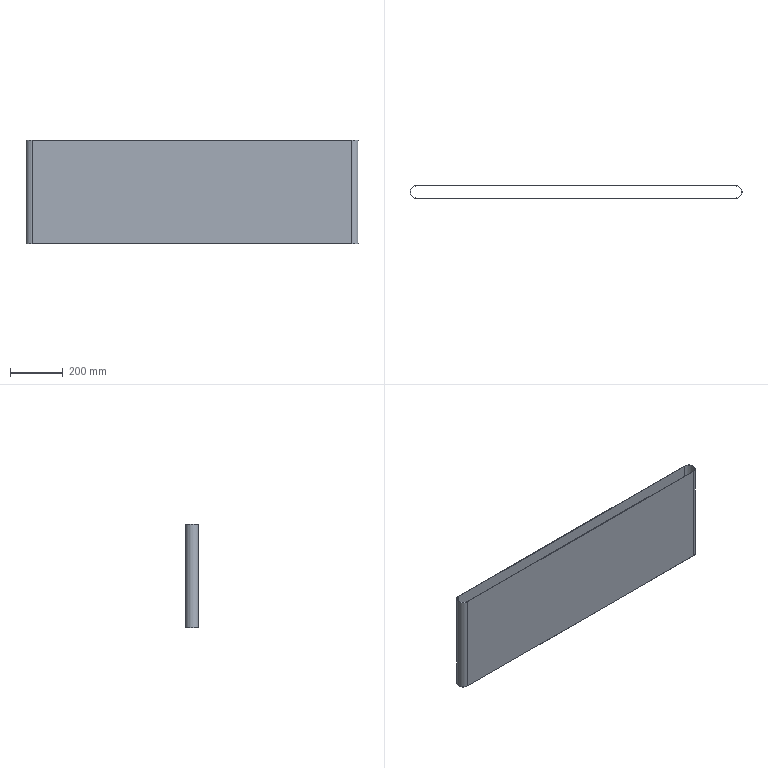Part | STEP file | RUBE509 | 1 solid | 10 faces | box 1253 x 49.2 x 390 mm | volume 1595905 mm3 | plane 6 | cylinder 4 | commonest cylinder face diameters 46 x2 49.2 x2
STEP:
#1=CARTESIAN_POINT('',(0.,0.,0.));
#2=DIRECTION('',(0.,0.,1.));
#3=DIRECTION('',(1.,0.,0.));
#4=AXIS2_PLACEMENT_3D('',#1,#2,#3);
#5=CARTESIAN_POINT('',(-1248.5,24.6,195.));
#6=VERTEX_POINT('',#5);
#7=CARTESIAN_POINT('',(-1248.5,-24.6,195.));
#8=VERTEX_POINT('',#7);
#9=CARTESIAN_POINT('',(-1248.5,0.,195.));
#10=DIRECTION('',(0.,0.,1.));
#11=DIRECTION('',(1.,0.,0.));
#12=AXIS2_PLACEMENT_3D('',#9,#10,#11);
#13=CIRCLE('',#12,24.6);
#14=CARTESIAN_POINT('',(-1248.5,0.,195.));
#15=DIRECTION('',(0.,0.,1.));
#16=DIRECTION('',(1.,0.,0.));
#17=AXIS2_PLACEMENT_3D('',#14,#15,#16);
#18=PLANE('',#17);
#19=CARTESIAN_POINT('',(0.,0.));
#20=DIRECTION('',(1.,0.));
#21=AXIS2_PLACEMENT_2D('',#19,#20);
#22=CIRCLE('',#21,24.6);
#23=(GEOMETRIC_REPRESENTATION_CONTEXT(2)PARAMETRIC_REPRESENTATION_CONTEXT()REPRESENTATION_CONTEXT('',''));
#24=DEFINITIONAL_REPRESENTATION('',(#22),#23);
#25=PCURVE('',#18,#24);
#26=CARTESIAN_POINT('',(-1248.5,0.,195.));
#27=DIRECTION('',(0.,0.,-1.));
#28=DIRECTION('',(-1.,0.,0.));
#29=AXIS2_PLACEMENT_3D('',#26,#27,#28);
#30=CYLINDRICAL_SURFACE('',#29,24.6);
#31=CARTESIAN_POINT('',(3.142,0.));
#32=DIRECTION('',(-1.,0.));
#33=VECTOR('',#32,1.);
#34=LINE('',#31,#33);
#35=(GEOMETRIC_REPRESENTATION_CONTEXT(2)PARAMETRIC_REPRESENTATION_CONTEXT()REPRESENTATION_CONTEXT('',''));
#36=DEFINITIONAL_REPRESENTATION('',(#34),#35);
#37=PCURVE('',#30,#36);
#38=SURFACE_CURVE('',#13,(#25,#37),.PCURVE_S1.);
#39=EDGE_CURVE('',#6,#8,#38,.T.);
#40=ORIENTED_EDGE('',*,*,#39,.T.);
#41=CARTESIAN_POINT('',(-44.5,-24.6,195.));
#42=VERTEX_POINT('',#41);
#43=CARTESIAN_POINT('',(-1248.5,-24.6,195.));
#44=DIRECTION('',(1.,0.,0.));
#45=VECTOR('',#44,1.);
#46=LINE('',#43,#45);
#47=CARTESIAN_POINT('',(0.,-24.6));
#48=DIRECTION('',(1.,0.));
#49=VECTOR('',#48,1.);
#50=LINE('',#47,#49);
#51=(GEOMETRIC_REPRESENTATION_CONTEXT(2)PARAMETRIC_REPRESENTATION_CONTEXT()REPRESENTATION_CONTEXT('',''));
#52=DEFINITIONAL_REPRESENTATION('',(#50),#51);
#53=PCURVE('',#18,#52);
#54=CARTESIAN_POINT('',(-1248.5,-24.6,195.));
#55=DIRECTION('',(0.,1.,0.));
#56=DIRECTION('',(-1.,0.,0.));
#57=AXIS2_PLACEMENT_3D('',#54,#55,#56);
#58=PLANE('',#57);
#59=CARTESIAN_POINT('',(0.,0.));
#60=DIRECTION('',(-1.,0.));
#61=VECTOR('',#60,1.);
#62=LINE('',#59,#61);
#63=(GEOMETRIC_REPRESENTATION_CONTEXT(2)PARAMETRIC_REPRESENTATION_CONTEXT()REPRESENTATION_CONTEXT('',''));
#64=DEFINITIONAL_REPRESENTATION('',(#62),#63);
#65=PCURVE('',#58,#64);
#66=SURFACE_CURVE('',#46,(#53,#65),.PCURVE_S1.);
#67=EDGE_CURVE('',#8,#42,#66,.T.);
#68=ORIENTED_EDGE('',*,*,#67,.T.);
#69=CARTESIAN_POINT('',(-44.5,24.6,195.));
#70=VERTEX_POINT('',#69);
#71=CARTESIAN_POINT('',(-44.5,0.,195.));
#72=DIRECTION('',(0.,0.,1.));
#73=DIRECTION('',(1.,0.,0.));
#74=AXIS2_PLACEMENT_3D('',#71,#72,#73);
#75=CIRCLE('',#74,24.6);
#76=CARTESIAN_POINT('',(1204.,0.));
#77=DIRECTION('',(1.,0.));
#78=AXIS2_PLACEMENT_2D('',#76,#77);
#79=CIRCLE('',#78,24.6);
#80=(GEOMETRIC_REPRESENTATION_CONTEXT(2)PARAMETRIC_REPRESENTATION_CONTEXT()REPRESENTATION_CONTEXT('',''));
#81=DEFINITIONAL_REPRESENTATION('',(#79),#80);
#82=PCURVE('',#18,#81);
#83=CARTESIAN_POINT('',(-44.5,0.,195.));
#84=DIRECTION('',(0.,0.,-1.));
#85=DIRECTION('',(-1.,0.,0.));
#86=AXIS2_PLACEMENT_3D('',#83,#84,#85);
#87=CYLINDRICAL_SURFACE('',#86,24.6);
#88=CARTESIAN_POINT('',(9.425,0.));
#89=DIRECTION('',(-1.,0.));
#90=VECTOR('',#89,1.);
#91=LINE('',#88,#90);
#92=(GEOMETRIC_REPRESENTATION_CONTEXT(2)PARAMETRIC_REPRESENTATION_CONTEXT()REPRESENTATION_CONTEXT('',''));
#93=DEFINITIONAL_REPRESENTATION('',(#91),#92);
#94=PCURVE('',#87,#93);
#95=SURFACE_CURVE('',#75,(#82,#94),.PCURVE_S1.);
#96=EDGE_CURVE('',#42,#70,#95,.T.);
#97=ORIENTED_EDGE('',*,*,#96,.T.);
#98=CARTESIAN_POINT('',(-1248.5,24.6,195.));
#99=DIRECTION('',(-1.,0.,0.));
#100=VECTOR('',#99,1.);
#101=LINE('',#98,#100);
#102=CARTESIAN_POINT('',(0.,24.6));
#103=DIRECTION('',(-1.,0.));
#104=VECTOR('',#103,1.);
#105=LINE('',#102,#104);
#106=(GEOMETRIC_REPRESENTATION_CONTEXT(2)PARAMETRIC_REPRESENTATION_CONTEXT()REPRESENTATION_CONTEXT('',''));
#107=DEFINITIONAL_REPRESENTATION('',(#105),#106);
#108=PCURVE('',#18,#107);
#109=CARTESIAN_POINT('',(-1248.5,24.6,195.));
#110=DIRECTION('',(0.,-1.,0.));
#111=DIRECTION('',(1.,0.,0.));
#112=AXIS2_PLACEMENT_3D('',#109,#110,#111);
#113=PLANE('',#112);
#114=CARTESIAN_POINT('',(0.,0.));
#115=DIRECTION('',(-1.,0.));
#116=VECTOR('',#115,1.);
#117=LINE('',#114,#116);
#118=(GEOMETRIC_REPRESENTATION_CONTEXT(2)PARAMETRIC_REPRESENTATION_CONTEXT()REPRESENTATION_CONTEXT('',''));
#119=DEFINITIONAL_REPRESENTATION('',(#117),#118);
#120=PCURVE('',#113,#119);
#121=SURFACE_CURVE('',#101,(#108,#120),.PCURVE_S1.);
#122=EDGE_CURVE('',#70,#6,#121,.T.);
#123=ORIENTED_EDGE('',*,*,#122,.T.);
#124=EDGE_LOOP('',(#40,#68,#97,#123));
#125=FACE_BOUND('',#124,.T.);
#126=CARTESIAN_POINT('',(-1248.5,-23.,195.));
#127=VERTEX_POINT('',#126);
#128=CARTESIAN_POINT('',(-44.5,-23.,195.));
#129=VERTEX_POINT('',#128);
#130=CARTESIAN_POINT('',(-1248.5,-23.,195.));
#131=DIRECTION('',(1.,0.,0.));
#132=VECTOR('',#131,1.);
#133=LINE('',#130,#132);
#134=CARTESIAN_POINT('',(0.,-23.));
#135=DIRECTION('',(1.,0.));
#136=VECTOR('',#135,1.);
#137=LINE('',#134,#136);
#138=(GEOMETRIC_REPRESENTATION_CONTEXT(2)PARAMETRIC_REPRESENTATION_CONTEXT()REPRESENTATION_CONTEXT('',''));
#139=DEFINITIONAL_REPRESENTATION('',(#137),#138);
#140=PCURVE('',#18,#139);
#141=CARTESIAN_POINT('',(-1248.5,-23.,195.));
#142=DIRECTION('',(0.,1.,0.));
#143=DIRECTION('',(-1.,0.,0.));
#144=AXIS2_PLACEMENT_3D('',#141,#142,#143);
#145=PLANE('',#144);
#146=CARTESIAN_POINT('',(0.,0.));
#147=DIRECTION('',(-1.,0.));
#148=VECTOR('',#147,1.);
#149=LINE('',#146,#148);
#150=(GEOMETRIC_REPRESENTATION_CONTEXT(2)PARAMETRIC_REPRESENTATION_CONTEXT()REPRESENTATION_CONTEXT('',''));
#151=DEFINITIONAL_REPRESENTATION('',(#149),#150);
#152=PCURVE('',#145,#151);
#153=SURFACE_CURVE('',#133,(#140,#152),.PCURVE_S1.);
#154=EDGE_CURVE('',#127,#129,#153,.T.);
#155=ORIENTED_EDGE('',*,*,#154,.F.);
#156=CARTESIAN_POINT('',(-1248.5,23.,195.));
#157=VERTEX_POINT('',#156);
#158=CARTESIAN_POINT('',(-1248.5,0.,195.));
#159=DIRECTION('',(0.,0.,1.));
#160=DIRECTION('',(1.,0.,0.));
#161=AXIS2_PLACEMENT_3D('',#158,#159,#160);
#162=CIRCLE('',#161,23.);
#163=CARTESIAN_POINT('',(0.,0.));
#164=DIRECTION('',(1.,0.));
#165=AXIS2_PLACEMENT_2D('',#163,#164);
#166=CIRCLE('',#165,23.);
#167=(GEOMETRIC_REPRESENTATION_CONTEXT(2)PARAMETRIC_REPRESENTATION_CONTEXT()REPRESENTATION_CONTEXT('',''));
#168=DEFINITIONAL_REPRESENTATION('',(#166),#167);
#169=PCURVE('',#18,#168);
#170=CARTESIAN_POINT('',(-1248.5,0.,195.));
#171=DIRECTION('',(0.,0.,-1.));
#172=DIRECTION('',(-1.,0.,0.));
#173=AXIS2_PLACEMENT_3D('',#170,#171,#172);
#174=CYLINDRICAL_SURFACE('',#173,23.);
#175=CARTESIAN_POINT('',(9.425,0.));
#176=DIRECTION('',(-1.,0.));
#177=VECTOR('',#176,1.);
#178=LINE('',#175,#177);
#179=(GEOMETRIC_REPRESENTATION_CONTEXT(2)PARAMETRIC_REPRESENTATION_CONTEXT()REPRESENTATION_CONTEXT('',''));
#180=DEFINITIONAL_REPRESENTATION('',(#178),#179);
#181=PCURVE('',#174,#180);
#182=SURFACE_CURVE('',#162,(#169,#181),.PCURVE_S1.);
#183=EDGE_CURVE('',#157,#127,#182,.T.);
#184=ORIENTED_EDGE('',*,*,#183,.F.);
#185=CARTESIAN_POINT('',(-44.5,23.,195.));
#186=VERTEX_POINT('',#185);
#187=CARTESIAN_POINT('',(-1248.5,23.,195.));
#188=DIRECTION('',(-1.,0.,0.));
#189=VECTOR('',#188,1.);
#190=LINE('',#187,#189);
#191=CARTESIAN_POINT('',(0.,23.));
#192=DIRECTION('',(-1.,0.));
#193=VECTOR('',#192,1.);
#194=LINE('',#191,#193);
#195=(GEOMETRIC_REPRESENTATION_CONTEXT(2)PARAMETRIC_REPRESENTATION_CONTEXT()REPRESENTATION_CONTEXT('',''));
#196=DEFINITIONAL_REPRESENTATION('',(#194),#195);
#197=PCURVE('',#18,#196);
#198=CARTESIAN_POINT('',(-1248.5,23.,195.));
#199=DIRECTION('',(0.,-1.,0.));
#200=DIRECTION('',(1.,0.,0.));
#201=AXIS2_PLACEMENT_3D('',#198,#199,#200);
#202=PLANE('',#201);
#203=CARTESIAN_POINT('',(0.,0.));
#204=DIRECTION('',(-1.,0.));
#205=VECTOR('',#204,1.);
#206=LINE('',#203,#205);
#207=(GEOMETRIC_REPRESENTATION_CONTEXT(2)PARAMETRIC_REPRESENTATION_CONTEXT()REPRESENTATION_CONTEXT('',''));
#208=DEFINITIONAL_REPRESENTATION('',(#206),#207);
#209=PCURVE('',#202,#208);
#210=SURFACE_CURVE('',#190,(#197,#209),.PCURVE_S1.);
#211=EDGE_CURVE('',#186,#157,#210,.T.);
#212=ORIENTED_EDGE('',*,*,#211,.F.);
#213=CARTESIAN_POINT('',(-44.5,0.,195.));
#214=DIRECTION('',(0.,0.,1.));
#215=DIRECTION('',(1.,0.,0.));
#216=AXIS2_PLACEMENT_3D('',#213,#214,#215);
#217=CIRCLE('',#216,23.);
#218=CARTESIAN_POINT('',(1204.,0.));
#219=DIRECTION('',(1.,0.));
#220=AXIS2_PLACEMENT_2D('',#218,#219);
#221=CIRCLE('',#220,23.);
#222=(GEOMETRIC_REPRESENTATION_CONTEXT(2)PARAMETRIC_REPRESENTATION_CONTEXT()REPRESENTATION_CONTEXT('',''));
#223=DEFINITIONAL_REPRESENTATION('',(#221),#222);
#224=PCURVE('',#18,#223);
#225=CARTESIAN_POINT('',(-44.5,0.,195.));
#226=DIRECTION('',(0.,0.,-1.));
#227=DIRECTION('',(-1.,0.,0.));
#228=AXIS2_PLACEMENT_3D('',#225,#226,#227);
#229=CYLINDRICAL_SURFACE('',#228,23.);
#230=CARTESIAN_POINT('',(9.425,0.));
#231=DIRECTION('',(-1.,0.));
#232=VECTOR('',#231,1.);
#233=LINE('',#230,#232);
#234=(GEOMETRIC_REPRESENTATION_CONTEXT(2)PARAMETRIC_REPRESENTATION_CONTEXT()REPRESENTATION_CONTEXT('',''));
#235=DEFINITIONAL_REPRESENTATION('',(#233),#234);
#236=PCURVE('',#229,#235);
#237=SURFACE_CURVE('',#217,(#224,#236),.PCURVE_S1.);
#238=EDGE_CURVE('',#129,#186,#237,.T.);
#239=ORIENTED_EDGE('',*,*,#238,.F.);
#240=EDGE_LOOP('',(#155,#184,#212,#239));
#241=FACE_BOUND('',#240,.T.);
#242=ADVANCED_FACE('',(#125,#241),#18,.T.);
#243=CARTESIAN_POINT('',(-1248.5,24.6,-195.));
#244=VERTEX_POINT('',#243);
#245=CARTESIAN_POINT('',(-1248.5,-24.6,-195.));
#246=VERTEX_POINT('',#245);
#247=CARTESIAN_POINT('',(-1248.5,0.,-195.));
#248=DIRECTION('',(0.,0.,1.));
#249=DIRECTION('',(1.,0.,0.));
#250=AXIS2_PLACEMENT_3D('',#247,#248,#249);
#251=CIRCLE('',#250,24.6);
#252=CARTESIAN_POINT('',(-1248.5,0.,-195.));
#253=DIRECTION('',(0.,0.,1.));
#254=DIRECTION('',(1.,0.,0.));
#255=AXIS2_PLACEMENT_3D('',#252,#253,#254);
#256=PLANE('',#255);
#257=CARTESIAN_POINT('',(0.,0.));
#258=DIRECTION('',(1.,0.));
#259=AXIS2_PLACEMENT_2D('',#257,#258);
#260=CIRCLE('',#259,24.6);
#261=(GEOMETRIC_REPRESENTATION_CONTEXT(2)PARAMETRIC_REPRESENTATION_CONTEXT()REPRESENTATION_CONTEXT('',''));
#262=DEFINITIONAL_REPRESENTATION('',(#260),#261);
#263=PCURVE('',#256,#262);
#264=CARTESIAN_POINT('',(3.142,390.));
#265=DIRECTION('',(-1.,0.));
#266=VECTOR('',#265,1.);
#267=LINE('',#264,#266);
#268=(GEOMETRIC_REPRESENTATION_CONTEXT(2)PARAMETRIC_REPRESENTATION_CONTEXT()REPRESENTATION_CONTEXT('',''));
#269=DEFINITIONAL_REPRESENTATION('',(#267),#268);
#270=PCURVE('',#30,#269);
#271=SURFACE_CURVE('',#251,(#263,#270),.PCURVE_S1.);
#272=EDGE_CURVE('',#244,#246,#271,.T.);
#273=ORIENTED_EDGE('',*,*,#272,.F.);
#274=CARTESIAN_POINT('',(-44.5,24.6,-195.));
#275=VERTEX_POINT('',#274);
#276=CARTESIAN_POINT('',(-1248.5,24.6,-195.));
#277=DIRECTION('',(-1.,0.,0.));
#278=VECTOR('',#277,1.);
#279=LINE('',#276,#278);
#280=CARTESIAN_POINT('',(0.,24.6));
#281=DIRECTION('',(-1.,0.));
#282=VECTOR('',#281,1.);
#283=LINE('',#280,#282);
#284=(GEOMETRIC_REPRESENTATION_CONTEXT(2)PARAMETRIC_REPRESENTATION_CONTEXT()REPRESENTATION_CONTEXT('',''));
#285=DEFINITIONAL_REPRESENTATION('',(#283),#284);
#286=PCURVE('',#256,#285);
#287=CARTESIAN_POINT('',(0.,-390.));
#288=DIRECTION('',(-1.,0.));
#289=VECTOR('',#288,1.);
#290=LINE('',#287,#289);
#291=(GEOMETRIC_REPRESENTATION_CONTEXT(2)PARAMETRIC_REPRESENTATION_CONTEXT()REPRESENTATION_CONTEXT('',''));
#292=DEFINITIONAL_REPRESENTATION('',(#290),#291);
#293=PCURVE('',#113,#292);
#294=SURFACE_CURVE('',#279,(#286,#293),.PCURVE_S1.);
#295=EDGE_CURVE('',#275,#244,#294,.T.);
#296=ORIENTED_EDGE('',*,*,#295,.F.);
#297=CARTESIAN_POINT('',(-44.5,-24.6,-195.));
#298=VERTEX_POINT('',#297);
#299=CARTESIAN_POINT('',(-44.5,0.,-195.));
#300=DIRECTION('',(0.,0.,1.));
#301=DIRECTION('',(1.,0.,0.));
#302=AXIS2_PLACEMENT_3D('',#299,#300,#301);
#303=CIRCLE('',#302,24.6);
#304=CARTESIAN_POINT('',(1204.,0.));
#305=DIRECTION('',(1.,0.));
#306=AXIS2_PLACEMENT_2D('',#304,#305);
#307=CIRCLE('',#306,24.6);
#308=(GEOMETRIC_REPRESENTATION_CONTEXT(2)PARAMETRIC_REPRESENTATION_CONTEXT()REPRESENTATION_CONTEXT('',''));
#309=DEFINITIONAL_REPRESENTATION('',(#307),#308);
#310=PCURVE('',#256,#309);
#311=CARTESIAN_POINT('',(9.425,390.));
#312=DIRECTION('',(-1.,0.));
#313=VECTOR('',#312,1.);
#314=LINE('',#311,#313);
#315=(GEOMETRIC_REPRESENTATION_CONTEXT(2)PARAMETRIC_REPRESENTATION_CONTEXT()REPRESENTATION_CONTEXT('',''));
#316=DEFINITIONAL_REPRESENTATION('',(#314),#315);
#317=PCURVE('',#87,#316);
#318=SURFACE_CURVE('',#303,(#310,#317),.PCURVE_S1.);
#319=EDGE_CURVE('',#298,#275,#318,.T.);
#320=ORIENTED_EDGE('',*,*,#319,.F.);
#321=CARTESIAN_POINT('',(-1248.5,-24.6,-195.));
#322=DIRECTION('',(1.,0.,0.));
#323=VECTOR('',#322,1.);
#324=LINE('',#321,#323);
#325=CARTESIAN_POINT('',(0.,-24.6));
#326=DIRECTION('',(1.,0.));
#327=VECTOR('',#326,1.);
#328=LINE('',#325,#327);
#329=(GEOMETRIC_REPRESENTATION_CONTEXT(2)PARAMETRIC_REPRESENTATION_CONTEXT()REPRESENTATION_CONTEXT('',''));
#330=DEFINITIONAL_REPRESENTATION('',(#328),#329);
#331=PCURVE('',#256,#330);
#332=CARTESIAN_POINT('',(0.,-390.));
#333=DIRECTION('',(-1.,0.));
#334=VECTOR('',#333,1.);
#335=LINE('',#332,#334);
#336=(GEOMETRIC_REPRESENTATION_CONTEXT(2)PARAMETRIC_REPRESENTATION_CONTEXT()REPRESENTATION_CONTEXT('',''));
#337=DEFINITIONAL_REPRESENTATION('',(#335),#336);
#338=PCURVE('',#58,#337);
#339=SURFACE_CURVE('',#324,(#331,#338),.PCURVE_S1.);
#340=EDGE_CURVE('',#246,#298,#339,.T.);
#341=ORIENTED_EDGE('',*,*,#340,.F.);
#342=EDGE_LOOP('',(#273,#296,#320,#341));
#343=FACE_BOUND('',#342,.T.);
#344=CARTESIAN_POINT('',(-1248.5,23.,-195.));
#345=VERTEX_POINT('',#344);
#346=CARTESIAN_POINT('',(-1248.5,-23.,-195.));
#347=VERTEX_POINT('',#346);
#348=CARTESIAN_POINT('',(-1248.5,0.,-195.));
#349=DIRECTION('',(0.,0.,1.));
#350=DIRECTION('',(1.,0.,0.));
#351=AXIS2_PLACEMENT_3D('',#348,#349,#350);
#352=CIRCLE('',#351,23.);
#353=CARTESIAN_POINT('',(0.,0.));
#354=DIRECTION('',(1.,0.));
#355=AXIS2_PLACEMENT_2D('',#353,#354);
#356=CIRCLE('',#355,23.);
#357=(GEOMETRIC_REPRESENTATION_CONTEXT(2)PARAMETRIC_REPRESENTATION_CONTEXT()REPRESENTATION_CONTEXT('',''));
#358=DEFINITIONAL_REPRESENTATION('',(#356),#357);
#359=PCURVE('',#256,#358);
#360=CARTESIAN_POINT('',(9.425,390.));
#361=DIRECTION('',(-1.,0.));
#362=VECTOR('',#361,1.);
#363=LINE('',#360,#362);
#364=(GEOMETRIC_REPRESENTATION_CONTEXT(2)PARAMETRIC_REPRESENTATION_CONTEXT()REPRESENTATION_CONTEXT('',''));
#365=DEFINITIONAL_REPRESENTATION('',(#363),#364);
#366=PCURVE('',#174,#365);
#367=SURFACE_CURVE('',#352,(#359,#366),.PCURVE_S1.);
#368=EDGE_CURVE('',#345,#347,#367,.T.);
#369=ORIENTED_EDGE('',*,*,#368,.T.);
#370=CARTESIAN_POINT('',(-44.5,-23.,-195.));
#371=VERTEX_POINT('',#370);
#372=CARTESIAN_POINT('',(-1248.5,-23.,-195.));
#373=DIRECTION('',(1.,0.,0.));
#374=VECTOR('',#373,1.);
#375=LINE('',#372,#374);
#376=CARTESIAN_POINT('',(0.,-23.));
#377=DIRECTION('',(1.,0.));
#378=VECTOR('',#377,1.);
#379=LINE('',#376,#378);
#380=(GEOMETRIC_REPRESENTATION_CONTEXT(2)PARAMETRIC_REPRESENTATION_CONTEXT()REPRESENTATION_CONTEXT('',''));
#381=DEFINITIONAL_REPRESENTATION('',(#379),#380);
#382=PCURVE('',#256,#381);
#383=CARTESIAN_POINT('',(0.,-390.));
#384=DIRECTION('',(-1.,0.));
#385=VECTOR('',#384,1.);
#386=LINE('',#383,#385);
#387=(GEOMETRIC_REPRESENTATION_CONTEXT(2)PARAMETRIC_REPRESENTATION_CONTEXT()REPRESENTATION_CONTEXT('',''));
#388=DEFINITIONAL_REPRESENTATION('',(#386),#387);
#389=PCURVE('',#145,#388);
#390=SURFACE_CURVE('',#375,(#382,#389),.PCURVE_S1.);
#391=EDGE_CURVE('',#347,#371,#390,.T.);
#392=ORIENTED_EDGE('',*,*,#391,.T.);
#393=CARTESIAN_POINT('',(-44.5,23.,-195.));
#394=VERTEX_POINT('',#393);
#395=CARTESIAN_POINT('',(-44.5,0.,-195.));
#396=DIRECTION('',(0.,0.,1.));
#397=DIRECTION('',(1.,0.,0.));
#398=AXIS2_PLACEMENT_3D('',#395,#396,#397);
#399=CIRCLE('',#398,23.);
#400=CARTESIAN_POINT('',(1204.,0.));
#401=DIRECTION('',(1.,0.));
#402=AXIS2_PLACEMENT_2D('',#400,#401);
#403=CIRCLE('',#402,23.);
#404=(GEOMETRIC_REPRESENTATION_CONTEXT(2)PARAMETRIC_REPRESENTATION_CONTEXT()REPRESENTATION_CONTEXT('',''));
#405=DEFINITIONAL_REPRESENTATION('',(#403),#404);
#406=PCURVE('',#256,#405);
#407=CARTESIAN_POINT('',(9.425,390.));
#408=DIRECTION('',(-1.,0.));
#409=VECTOR('',#408,1.);
#410=LINE('',#407,#409);
#411=(GEOMETRIC_REPRESENTATION_CONTEXT(2)PARAMETRIC_REPRESENTATION_CONTEXT()REPRESENTATION_CONTEXT('',''));
#412=DEFINITIONAL_REPRESENTATION('',(#410),#411);
#413=PCURVE('',#229,#412);
#414=SURFACE_CURVE('',#399,(#406,#413),.PCURVE_S1.);
#415=EDGE_CURVE('',#371,#394,#414,.T.);
#416=ORIENTED_EDGE('',*,*,#415,.T.);
#417=CARTESIAN_POINT('',(-1248.5,23.,-195.));
#418=DIRECTION('',(-1.,0.,0.));
#419=VECTOR('',#418,1.);
#420=LINE('',#417,#419);
#421=CARTESIAN_POINT('',(0.,23.));
#422=DIRECTION('',(-1.,0.));
#423=VECTOR('',#422,1.);
#424=LINE('',#421,#423);
#425=(GEOMETRIC_REPRESENTATION_CONTEXT(2)PARAMETRIC_REPRESENTATION_CONTEXT()REPRESENTATION_CONTEXT('',''));
#426=DEFINITIONAL_REPRESENTATION('',(#424),#425);
#427=PCURVE('',#256,#426);
#428=CARTESIAN_POINT('',(0.,-390.));
#429=DIRECTION('',(-1.,0.));
#430=VECTOR('',#429,1.);
#431=LINE('',#428,#430);
#432=(GEOMETRIC_REPRESENTATION_CONTEXT(2)PARAMETRIC_REPRESENTATION_CONTEXT()REPRESENTATION_CONTEXT('',''));
#433=DEFINITIONAL_REPRESENTATION('',(#431),#432);
#434=PCURVE('',#202,#433);
#435=SURFACE_CURVE('',#420,(#427,#434),.PCURVE_S1.);
#436=EDGE_CURVE('',#394,#345,#435,.T.);
#437=ORIENTED_EDGE('',*,*,#436,.T.);
#438=EDGE_LOOP('',(#369,#392,#416,#437));
#439=FACE_BOUND('',#438,.T.);
#440=ADVANCED_FACE('',(#343,#439),#256,.F.);
#441=ORIENTED_EDGE('',*,*,#272,.T.);
#442=CARTESIAN_POINT('',(-1248.5,-24.6,195.));
#443=DIRECTION('',(0.,0.,-1.));
#444=VECTOR('',#443,1.);
#445=LINE('',#442,#444);
#446=CARTESIAN_POINT('',(-1.571,0.));
#447=DIRECTION('',(0.,1.));
#448=VECTOR('',#447,1.);
#449=LINE('',#446,#448);
#450=(GEOMETRIC_REPRESENTATION_CONTEXT(2)PARAMETRIC_REPRESENTATION_CONTEXT()REPRESENTATION_CONTEXT('',''));
#451=DEFINITIONAL_REPRESENTATION('',(#449),#450);
#452=PCURVE('',#30,#451);
#453=CARTESIAN_POINT('',(0.,0.));
#454=DIRECTION('',(0.,-1.));
#455=VECTOR('',#454,1.);
#456=LINE('',#453,#455);
#457=(GEOMETRIC_REPRESENTATION_CONTEXT(2)PARAMETRIC_REPRESENTATION_CONTEXT()REPRESENTATION_CONTEXT('',''));
#458=DEFINITIONAL_REPRESENTATION('',(#456),#457);
#459=PCURVE('',#58,#458);
#460=SURFACE_CURVE('',#445,(#452,#459),.PCURVE_S1.);
#461=EDGE_CURVE('',#8,#246,#460,.T.);
#462=ORIENTED_EDGE('',*,*,#461,.F.);
#463=ORIENTED_EDGE('',*,*,#39,.F.);
#464=CARTESIAN_POINT('',(-1248.5,24.6,195.));
#465=DIRECTION('',(0.,0.,-1.));
#466=VECTOR('',#465,1.);
#467=LINE('',#464,#466);
#468=CARTESIAN_POINT('',(1.571,0.));
#469=DIRECTION('',(0.,1.));
#470=VECTOR('',#469,1.);
#471=LINE('',#468,#470);
#472=(GEOMETRIC_REPRESENTATION_CONTEXT(2)PARAMETRIC_REPRESENTATION_CONTEXT()REPRESENTATION_CONTEXT('',''));
#473=DEFINITIONAL_REPRESENTATION('',(#471),#472);
#474=PCURVE('',#30,#473);
#475=CARTESIAN_POINT('',(0.,0.));
#476=DIRECTION('',(0.,-1.));
#477=VECTOR('',#476,1.);
#478=LINE('',#475,#477);
#479=(GEOMETRIC_REPRESENTATION_CONTEXT(2)PARAMETRIC_REPRESENTATION_CONTEXT()REPRESENTATION_CONTEXT('',''));
#480=DEFINITIONAL_REPRESENTATION('',(#478),#479);
#481=PCURVE('',#113,#480);
#482=SURFACE_CURVE('',#467,(#474,#481),.PCURVE_S1.);
#483=EDGE_CURVE('',#6,#244,#482,.T.);
#484=ORIENTED_EDGE('',*,*,#483,.T.);
#485=EDGE_LOOP('',(#441,#462,#463,#484));
#486=FACE_BOUND('',#485,.T.);
#487=ADVANCED_FACE('',(#486),#30,.T.);
#488=ORIENTED_EDGE('',*,*,#340,.T.);
#489=CARTESIAN_POINT('',(-44.5,-24.6,195.));
#490=DIRECTION('',(0.,0.,-1.));
#491=VECTOR('',#490,1.);
#492=LINE('',#489,#491);
#493=CARTESIAN_POINT('',(-1204.,0.));
#494=DIRECTION('',(0.,-1.));
#495=VECTOR('',#494,1.);
#496=LINE('',#493,#495);
#497=(GEOMETRIC_REPRESENTATION_CONTEXT(2)PARAMETRIC_REPRESENTATION_CONTEXT()REPRESENTATION_CONTEXT('',''));
#498=DEFINITIONAL_REPRESENTATION('',(#496),#497);
#499=PCURVE('',#58,#498);
#500=CARTESIAN_POINT('',(4.712,0.));
#501=DIRECTION('',(0.,1.));
#502=VECTOR('',#501,1.);
#503=LINE('',#500,#502);
#504=(GEOMETRIC_REPRESENTATION_CONTEXT(2)PARAMETRIC_REPRESENTATION_CONTEXT()REPRESENTATION_CONTEXT('',''));
#505=DEFINITIONAL_REPRESENTATION('',(#503),#504);
#506=PCURVE('',#87,#505);
#507=SURFACE_CURVE('',#492,(#499,#506),.PCURVE_S1.);
#508=EDGE_CURVE('',#42,#298,#507,.T.);
#509=ORIENTED_EDGE('',*,*,#508,.F.);
#510=ORIENTED_EDGE('',*,*,#67,.F.);
#511=ORIENTED_EDGE('',*,*,#461,.T.);
#512=EDGE_LOOP('',(#488,#509,#510,#511));
#513=FACE_BOUND('',#512,.T.);
#514=ADVANCED_FACE('',(#513),#58,.F.);
#515=ORIENTED_EDGE('',*,*,#319,.T.);
#516=CARTESIAN_POINT('',(-44.5,24.6,195.));
#517=DIRECTION('',(0.,0.,-1.));
#518=VECTOR('',#517,1.);
#519=LINE('',#516,#518);
#520=CARTESIAN_POINT('',(1.571,0.));
#521=DIRECTION('',(0.,1.));
#522=VECTOR('',#521,1.);
#523=LINE('',#520,#522);
#524=(GEOMETRIC_REPRESENTATION_CONTEXT(2)PARAMETRIC_REPRESENTATION_CONTEXT()REPRESENTATION_CONTEXT('',''));
#525=DEFINITIONAL_REPRESENTATION('',(#523),#524);
#526=PCURVE('',#87,#525);
#527=CARTESIAN_POINT('',(1204.,0.));
#528=DIRECTION('',(0.,-1.));
#529=VECTOR('',#528,1.);
#530=LINE('',#527,#529);
#531=(GEOMETRIC_REPRESENTATION_CONTEXT(2)PARAMETRIC_REPRESENTATION_CONTEXT()REPRESENTATION_CONTEXT('',''));
#532=DEFINITIONAL_REPRESENTATION('',(#530),#531);
#533=PCURVE('',#113,#532);
#534=SURFACE_CURVE('',#519,(#526,#533),.PCURVE_S1.);
#535=EDGE_CURVE('',#70,#275,#534,.T.);
#536=ORIENTED_EDGE('',*,*,#535,.F.);
#537=ORIENTED_EDGE('',*,*,#96,.F.);
#538=ORIENTED_EDGE('',*,*,#508,.T.);
#539=EDGE_LOOP('',(#515,#536,#537,#538));
#540=FACE_BOUND('',#539,.T.);
#541=ADVANCED_FACE('',(#540),#87,.T.);
#542=ORIENTED_EDGE('',*,*,#295,.T.);
#543=ORIENTED_EDGE('',*,*,#483,.F.);
#544=ORIENTED_EDGE('',*,*,#122,.F.);
#545=ORIENTED_EDGE('',*,*,#535,.T.);
#546=EDGE_LOOP('',(#542,#543,#544,#545));
#547=FACE_BOUND('',#546,.T.);
#548=ADVANCED_FACE('',(#547),#113,.F.);
#549=CARTESIAN_POINT('',(-1248.5,-23.,195.));
#550=DIRECTION('',(0.,0.,-1.));
#551=VECTOR('',#550,1.);
#552=LINE('',#549,#551);
#553=CARTESIAN_POINT('',(4.712,0.));
#554=DIRECTION('',(0.,1.));
#555=VECTOR('',#554,1.);
#556=LINE('',#553,#555);
#557=(GEOMETRIC_REPRESENTATION_CONTEXT(2)PARAMETRIC_REPRESENTATION_CONTEXT()REPRESENTATION_CONTEXT('',''));
#558=DEFINITIONAL_REPRESENTATION('',(#556),#557);
#559=PCURVE('',#174,#558);
#560=CARTESIAN_POINT('',(0.,0.));
#561=DIRECTION('',(0.,-1.));
#562=VECTOR('',#561,1.);
#563=LINE('',#560,#562);
#564=(GEOMETRIC_REPRESENTATION_CONTEXT(2)PARAMETRIC_REPRESENTATION_CONTEXT()REPRESENTATION_CONTEXT('',''));
#565=DEFINITIONAL_REPRESENTATION('',(#563),#564);
#566=PCURVE('',#145,#565);
#567=SURFACE_CURVE('',#552,(#559,#566),.PCURVE_S1.);
#568=EDGE_CURVE('',#127,#347,#567,.T.);
#569=ORIENTED_EDGE('',*,*,#568,.F.);
#570=ORIENTED_EDGE('',*,*,#183,.F.);
#571=CARTESIAN_POINT('',(-1248.5,23.,195.));
#572=DIRECTION('',(0.,0.,-1.));
#573=VECTOR('',#572,1.);
#574=LINE('',#571,#573);
#575=CARTESIAN_POINT('',(7.854,0.));
#576=DIRECTION('',(0.,1.));
#577=VECTOR('',#576,1.);
#578=LINE('',#575,#577);
#579=(GEOMETRIC_REPRESENTATION_CONTEXT(2)PARAMETRIC_REPRESENTATION_CONTEXT()REPRESENTATION_CONTEXT('',''));
#580=DEFINITIONAL_REPRESENTATION('',(#578),#579);
#581=PCURVE('',#174,#580);
#582=CARTESIAN_POINT('',(0.,0.));
#583=DIRECTION('',(0.,-1.));
#584=VECTOR('',#583,1.);
#585=LINE('',#582,#584);
#586=(GEOMETRIC_REPRESENTATION_CONTEXT(2)PARAMETRIC_REPRESENTATION_CONTEXT()REPRESENTATION_CONTEXT('',''));
#587=DEFINITIONAL_REPRESENTATION('',(#585),#586);
#588=PCURVE('',#202,#587);
#589=SURFACE_CURVE('',#574,(#581,#588),.PCURVE_S1.);
#590=EDGE_CURVE('',#157,#345,#589,.T.);
#591=ORIENTED_EDGE('',*,*,#590,.T.);
#592=ORIENTED_EDGE('',*,*,#368,.T.);
#593=EDGE_LOOP('',(#569,#570,#591,#592));
#594=FACE_BOUND('',#593,.F.);
#595=ADVANCED_FACE('',(#594),#174,.F.);
#596=ORIENTED_EDGE('',*,*,#391,.F.);
#597=ORIENTED_EDGE('',*,*,#568,.F.);
#598=ORIENTED_EDGE('',*,*,#154,.T.);
#599=CARTESIAN_POINT('',(-44.5,-23.,195.));
#600=DIRECTION('',(0.,0.,-1.));
#601=VECTOR('',#600,1.);
#602=LINE('',#599,#601);
#603=CARTESIAN_POINT('',(-1204.,0.));
#604=DIRECTION('',(0.,-1.));
#605=VECTOR('',#604,1.);
#606=LINE('',#603,#605);
#607=(GEOMETRIC_REPRESENTATION_CONTEXT(2)PARAMETRIC_REPRESENTATION_CONTEXT()REPRESENTATION_CONTEXT('',''));
#608=DEFINITIONAL_REPRESENTATION('',(#606),#607);
#609=PCURVE('',#145,#608);
#610=CARTESIAN_POINT('',(4.712,0.));
#611=DIRECTION('',(0.,1.));
#612=VECTOR('',#611,1.);
#613=LINE('',#610,#612);
#614=(GEOMETRIC_REPRESENTATION_CONTEXT(2)PARAMETRIC_REPRESENTATION_CONTEXT()REPRESENTATION_CONTEXT('',''));
#615=DEFINITIONAL_REPRESENTATION('',(#613),#614);
#616=PCURVE('',#229,#615);
#617=SURFACE_CURVE('',#602,(#609,#616),.PCURVE_S1.);
#618=EDGE_CURVE('',#129,#371,#617,.T.);
#619=ORIENTED_EDGE('',*,*,#618,.T.);
#620=EDGE_LOOP('',(#596,#597,#598,#619));
#621=FACE_BOUND('',#620,.T.);
#622=ADVANCED_FACE('',(#621),#145,.T.);
#623=CARTESIAN_POINT('',(-44.5,23.,195.));
#624=DIRECTION('',(0.,0.,-1.));
#625=VECTOR('',#624,1.);
#626=LINE('',#623,#625);
#627=CARTESIAN_POINT('',(1.571,0.));
#628=DIRECTION('',(0.,1.));
#629=VECTOR('',#628,1.);
#630=LINE('',#627,#629);
#631=(GEOMETRIC_REPRESENTATION_CONTEXT(2)PARAMETRIC_REPRESENTATION_CONTEXT()REPRESENTATION_CONTEXT('',''));
#632=DEFINITIONAL_REPRESENTATION('',(#630),#631);
#633=PCURVE('',#229,#632);
#634=CARTESIAN_POINT('',(1204.,0.));
#635=DIRECTION('',(0.,-1.));
#636=VECTOR('',#635,1.);
#637=LINE('',#634,#636);
#638=(GEOMETRIC_REPRESENTATION_CONTEXT(2)PARAMETRIC_REPRESENTATION_CONTEXT()REPRESENTATION_CONTEXT('',''));
#639=DEFINITIONAL_REPRESENTATION('',(#637),#638);
#640=PCURVE('',#202,#639);
#641=SURFACE_CURVE('',#626,(#633,#640),.PCURVE_S1.);
#642=EDGE_CURVE('',#186,#394,#641,.T.);
#643=ORIENTED_EDGE('',*,*,#642,.F.);
#644=ORIENTED_EDGE('',*,*,#238,.F.);
#645=ORIENTED_EDGE('',*,*,#618,.T.);
#646=ORIENTED_EDGE('',*,*,#415,.T.);
#647=EDGE_LOOP('',(#643,#644,#645,#646));
#648=FACE_BOUND('',#647,.F.);
#649=ADVANCED_FACE('',(#648),#229,.F.);
#650=ORIENTED_EDGE('',*,*,#436,.F.);
#651=ORIENTED_EDGE('',*,*,#642,.F.);
#652=ORIENTED_EDGE('',*,*,#211,.T.);
#653=ORIENTED_EDGE('',*,*,#590,.T.);
#654=EDGE_LOOP('',(#650,#651,#652,#653));
#655=FACE_BOUND('',#654,.T.);
#656=ADVANCED_FACE('',(#655),#202,.T.);
#657=CLOSED_SHELL('',(#242,#440,#487,#514,#541,#548,#595,#622,#649,#656));
#658=MANIFOLD_SOLID_BREP('',#657);
#659=(LENGTH_UNIT()NAMED_UNIT(*)SI_UNIT(.MILLI.,.METRE.));
#660=UNCERTAINTY_MEASURE_WITH_UNIT(LENGTH_MEASURE(0.0000001),#659,'','');
#661=(NAMED_UNIT(*)PLANE_ANGLE_UNIT()SI_UNIT($,.RADIAN.));
#662=(NAMED_UNIT(*)SI_UNIT($,.STERADIAN.)SOLID_ANGLE_UNIT());
#663=(GEOMETRIC_REPRESENTATION_CONTEXT(3)GLOBAL_UNCERTAINTY_ASSIGNED_CONTEXT((#660))GLOBAL_UNIT_ASSIGNED_CONTEXT((#659,#661,#662))REPRESENTATION_CONTEXT('',''));
#664=ADVANCED_BREP_SHAPE_REPRESENTATION('',(#4,#658),#663);